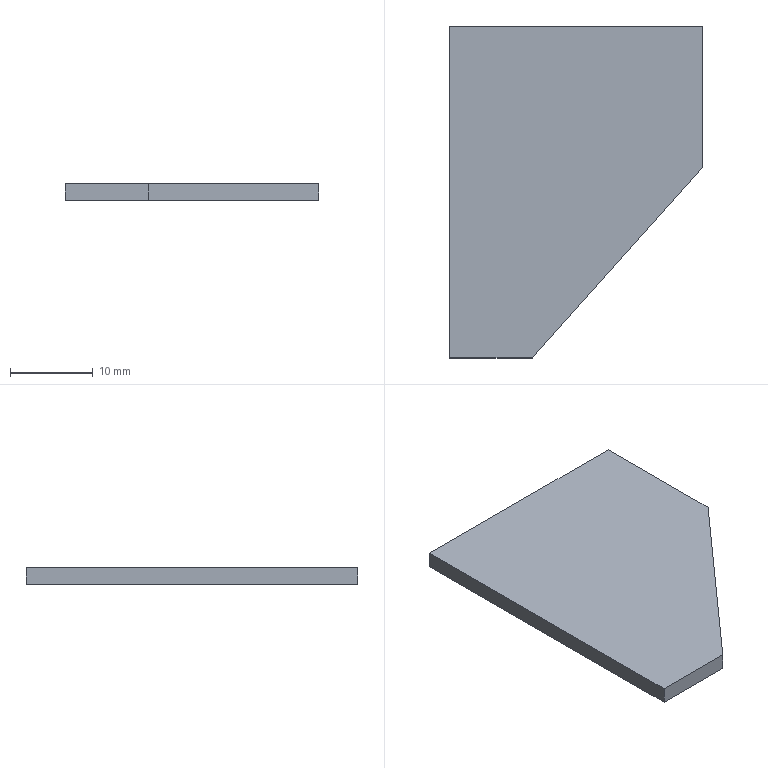Part | SolidWorks | features Extrusion 1 | 1 solid | 7 faces | box 30.5 x 40 x 2 mm | volume 1968 mm3 | plane 7
STEP:
#1=CARTESIAN_POINT('',(0.,0.,0.));
#2=VERTEX_POINT('',#1);
#3=CARTESIAN_POINT('',(0.,-40.,0.));
#4=VERTEX_POINT('',#3);
#5=CARTESIAN_POINT('',(0.,-40.,0.));
#6=DIRECTION('',(0.,-1.,0.));
#7=VECTOR('',#6,1000.);
#8=LINE('',#5,#7);
#9=EDGE_CURVE('',#2,#4,#8,.T.);
#10=ORIENTED_EDGE('',*,*,#9,.T.);
#11=CARTESIAN_POINT('',(0.,-40.,2.));
#12=VERTEX_POINT('',#11);
#13=CARTESIAN_POINT('',(0.,-40.,2.));
#14=DIRECTION('',(0.,0.,-1.));
#15=VECTOR('',#14,1000.);
#16=LINE('',#13,#15);
#17=EDGE_CURVE('',#12,#4,#16,.T.);
#18=ORIENTED_EDGE('',*,*,#17,.F.);
#19=CARTESIAN_POINT('',(0.,0.,2.));
#20=VERTEX_POINT('',#19);
#21=CARTESIAN_POINT('',(0.,-40.,2.));
#22=DIRECTION('',(0.,-1.,0.));
#23=VECTOR('',#22,1000.);
#24=LINE('',#21,#23);
#25=EDGE_CURVE('',#20,#12,#24,.T.);
#26=ORIENTED_EDGE('',*,*,#25,.F.);
#27=CARTESIAN_POINT('',(0.,0.,2.));
#28=DIRECTION('',(0.,0.,-1.));
#29=VECTOR('',#28,1000.);
#30=LINE('',#27,#29);
#31=EDGE_CURVE('',#20,#2,#30,.T.);
#32=ORIENTED_EDGE('',*,*,#31,.T.);
#33=EDGE_LOOP('',(#10,#18,#26,#32));
#34=FACE_OUTER_BOUND('',#33,.T.);
#35=CARTESIAN_POINT('',(0.,-40.,2.));
#36=DIRECTION('',(1.,0.,0.));
#37=DIRECTION('',(0.,0.,-1.));
#38=AXIS2_PLACEMENT_3D('',#35,#36,#37);
#39=PLANE('',#38);
#40=ADVANCED_FACE('',(#34),#39,.F.);
#41=CARTESIAN_POINT('',(10.,-40.,0.));
#42=VERTEX_POINT('',#41);
#43=CARTESIAN_POINT('',(10.,-40.,0.));
#44=DIRECTION('',(1.,0.,0.));
#45=VECTOR('',#44,1000.);
#46=LINE('',#43,#45);
#47=EDGE_CURVE('',#4,#42,#46,.T.);
#48=ORIENTED_EDGE('',*,*,#47,.T.);
#49=CARTESIAN_POINT('',(10.,-40.,2.));
#50=VERTEX_POINT('',#49);
#51=CARTESIAN_POINT('',(10.,-40.,2.));
#52=DIRECTION('',(0.,0.,-1.));
#53=VECTOR('',#52,1000.);
#54=LINE('',#51,#53);
#55=EDGE_CURVE('',#50,#42,#54,.T.);
#56=ORIENTED_EDGE('',*,*,#55,.F.);
#57=CARTESIAN_POINT('',(10.,-40.,2.));
#58=DIRECTION('',(1.,0.,0.));
#59=VECTOR('',#58,1000.);
#60=LINE('',#57,#59);
#61=EDGE_CURVE('',#12,#50,#60,.T.);
#62=ORIENTED_EDGE('',*,*,#61,.F.);
#63=ORIENTED_EDGE('',*,*,#17,.T.);
#64=EDGE_LOOP('',(#48,#56,#62,#63));
#65=FACE_OUTER_BOUND('',#64,.T.);
#66=CARTESIAN_POINT('',(10.,-40.,2.));
#67=DIRECTION('',(0.,1.,0.));
#68=DIRECTION('',(0.,0.,1.));
#69=AXIS2_PLACEMENT_3D('',#66,#67,#68);
#70=PLANE('',#69);
#71=ADVANCED_FACE('',(#65),#70,.F.);
#72=CARTESIAN_POINT('',(30.5,-17.,0.));
#73=VERTEX_POINT('',#72);
#74=CARTESIAN_POINT('',(30.5,-17.,0.));
#75=DIRECTION('',(0.6654,0.7465,0.));
#76=VECTOR('',#75,1000.);
#77=LINE('',#74,#76);
#78=EDGE_CURVE('',#42,#73,#77,.T.);
#79=ORIENTED_EDGE('',*,*,#78,.T.);
#80=CARTESIAN_POINT('',(30.5,-17.,2.));
#81=VERTEX_POINT('',#80);
#82=CARTESIAN_POINT('',(30.5,-17.,2.));
#83=DIRECTION('',(0.,0.,-1.));
#84=VECTOR('',#83,1000.);
#85=LINE('',#82,#84);
#86=EDGE_CURVE('',#81,#73,#85,.T.);
#87=ORIENTED_EDGE('',*,*,#86,.F.);
#88=CARTESIAN_POINT('',(30.5,-17.,2.));
#89=DIRECTION('',(0.6654,0.7465,0.));
#90=VECTOR('',#89,1000.);
#91=LINE('',#88,#90);
#92=EDGE_CURVE('',#50,#81,#91,.T.);
#93=ORIENTED_EDGE('',*,*,#92,.F.);
#94=ORIENTED_EDGE('',*,*,#55,.T.);
#95=EDGE_LOOP('',(#79,#87,#93,#94));
#96=FACE_OUTER_BOUND('',#95,.T.);
#97=CARTESIAN_POINT('',(30.5,-17.,2.));
#98=DIRECTION('',(-0.7465,0.6654,0.));
#99=DIRECTION('',(-0.6654,-0.7465,0.));
#100=AXIS2_PLACEMENT_3D('',#97,#98,#99);
#101=PLANE('',#100);
#102=ADVANCED_FACE('',(#96),#101,.F.);
#103=CARTESIAN_POINT('',(30.5,0.,0.));
#104=VERTEX_POINT('',#103);
#105=CARTESIAN_POINT('',(30.5,0.,0.));
#106=DIRECTION('',(0.,1.,0.));
#107=VECTOR('',#106,1000.);
#108=LINE('',#105,#107);
#109=EDGE_CURVE('',#73,#104,#108,.T.);
#110=ORIENTED_EDGE('',*,*,#109,.T.);
#111=CARTESIAN_POINT('',(30.5,0.,2.));
#112=VERTEX_POINT('',#111);
#113=CARTESIAN_POINT('',(30.5,0.,2.));
#114=DIRECTION('',(0.,0.,-1.));
#115=VECTOR('',#114,1000.);
#116=LINE('',#113,#115);
#117=EDGE_CURVE('',#112,#104,#116,.T.);
#118=ORIENTED_EDGE('',*,*,#117,.F.);
#119=CARTESIAN_POINT('',(30.5,0.,2.));
#120=DIRECTION('',(0.,1.,0.));
#121=VECTOR('',#120,1000.);
#122=LINE('',#119,#121);
#123=EDGE_CURVE('',#81,#112,#122,.T.);
#124=ORIENTED_EDGE('',*,*,#123,.F.);
#125=ORIENTED_EDGE('',*,*,#86,.T.);
#126=EDGE_LOOP('',(#110,#118,#124,#125));
#127=FACE_OUTER_BOUND('',#126,.T.);
#128=CARTESIAN_POINT('',(30.5,0.,2.));
#129=DIRECTION('',(-1.,0.,0.));
#130=DIRECTION('',(0.,-1.,0.));
#131=AXIS2_PLACEMENT_3D('',#128,#129,#130);
#132=PLANE('',#131);
#133=ADVANCED_FACE('',(#127),#132,.F.);
#134=CARTESIAN_POINT('',(0.,0.,0.));
#135=DIRECTION('',(-1.,0.,0.));
#136=VECTOR('',#135,1000.);
#137=LINE('',#134,#136);
#138=EDGE_CURVE('',#104,#2,#137,.T.);
#139=ORIENTED_EDGE('',*,*,#138,.T.);
#140=ORIENTED_EDGE('',*,*,#31,.F.);
#141=CARTESIAN_POINT('',(0.,0.,2.));
#142=DIRECTION('',(-1.,0.,0.));
#143=VECTOR('',#142,1000.);
#144=LINE('',#141,#143);
#145=EDGE_CURVE('',#112,#20,#144,.T.);
#146=ORIENTED_EDGE('',*,*,#145,.F.);
#147=ORIENTED_EDGE('',*,*,#117,.T.);
#148=EDGE_LOOP('',(#139,#140,#146,#147));
#149=FACE_OUTER_BOUND('',#148,.T.);
#150=CARTESIAN_POINT('',(0.,0.,2.));
#151=DIRECTION('',(0.,-1.,0.));
#152=DIRECTION('',(0.,0.,-1.));
#153=AXIS2_PLACEMENT_3D('',#150,#151,#152);
#154=PLANE('',#153);
#155=ADVANCED_FACE('',(#149),#154,.F.);
#156=ORIENTED_EDGE('',*,*,#25,.T.);
#157=ORIENTED_EDGE('',*,*,#61,.T.);
#158=ORIENTED_EDGE('',*,*,#92,.T.);
#159=ORIENTED_EDGE('',*,*,#123,.T.);
#160=ORIENTED_EDGE('',*,*,#145,.T.);
#161=EDGE_LOOP('',(#156,#157,#158,#159,#160));
#162=FACE_OUTER_BOUND('',#161,.T.);
#163=CARTESIAN_POINT('',(0.,0.,2.));
#164=DIRECTION('',(0.,0.,-1.));
#165=DIRECTION('',(-1.,0.,0.));
#166=AXIS2_PLACEMENT_3D('',#163,#164,#165);
#167=PLANE('',#166);
#168=ADVANCED_FACE('',(#162),#167,.F.);
#169=ORIENTED_EDGE('',*,*,#9,.F.);
#170=ORIENTED_EDGE('',*,*,#138,.F.);
#171=ORIENTED_EDGE('',*,*,#109,.F.);
#172=ORIENTED_EDGE('',*,*,#78,.F.);
#173=ORIENTED_EDGE('',*,*,#47,.F.);
#174=EDGE_LOOP('',(#169,#170,#171,#172,#173));
#175=FACE_OUTER_BOUND('',#174,.T.);
#176=CARTESIAN_POINT('',(0.,0.,0.));
#177=DIRECTION('',(0.,0.,-1.));
#178=DIRECTION('',(-1.,0.,0.));
#179=AXIS2_PLACEMENT_3D('',#176,#177,#178);
#180=PLANE('',#179);
#181=ADVANCED_FACE('',(#175),#180,.T.);
#182=CLOSED_SHELL('',(#40,#71,#102,#133,#155,#168,#181));
#183=MANIFOLD_SOLID_BREP('',#182);
#184=CARTESIAN_POINT('',(0.,0.,0.));
#185=DIRECTION('',(0.,0.,1.));
#186=DIRECTION('',(1.,0.,0.));
#187=AXIS2_PLACEMENT_3D('',#184,#185,#186);
#188=(LENGTH_UNIT()NAMED_UNIT(*)SI_UNIT(.MILLI.,.METRE.));
#189=UNCERTAINTY_MEASURE_WITH_UNIT(LENGTH_MEASURE(0.00001),#188,'','');
#190=(NAMED_UNIT(*)PLANE_ANGLE_UNIT()SI_UNIT($,.RADIAN.));
#191=(NAMED_UNIT(*)SI_UNIT($,.STERADIAN.)SOLID_ANGLE_UNIT());
#192=(GEOMETRIC_REPRESENTATION_CONTEXT(3)GLOBAL_UNCERTAINTY_ASSIGNED_CONTEXT((#189))GLOBAL_UNIT_ASSIGNED_CONTEXT((#188,#190,#191))REPRESENTATION_CONTEXT('',''));
#193=ADVANCED_BREP_SHAPE_REPRESENTATION('',(#183,#187),#192);